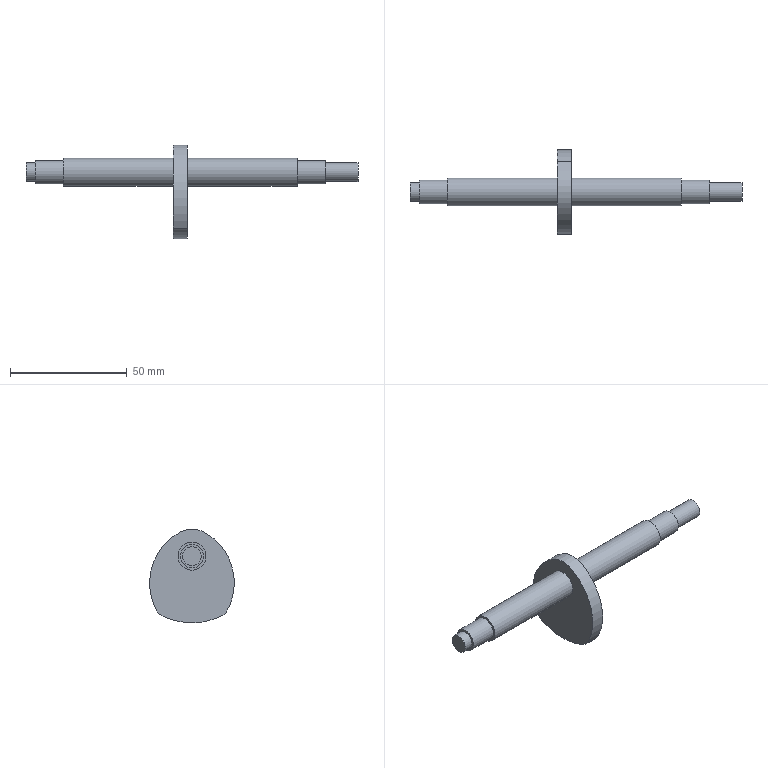Part | NX | features DATUM_CSYS 2, EXTRUDE 1, SKETCH 1, SWP104 1 | 1 solid | 16 faces | box 142 x 36.204 x 40.001 mm | volume 20323 mm3 | plane 8 | cylinder 6 | spline 2 | commonest cylinder face diameters 8 x2 10 x2 12 x2
STEP:
#1=CARTESIAN_POINT('',(-71.,0.,4.));
#2=VERTEX_POINT('',#1);
#3=CARTESIAN_POINT('',(-71.,0.,0.));
#4=DIRECTION('',(-1.,0.,0.));
#5=DIRECTION('',(0.,0.,1.));
#6=AXIS2_PLACEMENT_3D('',#3,#4,#5);
#7=CIRCLE('',#6,4.);
#8=EDGE_CURVE('',#2,#2,#7,.T.);
#9=ORIENTED_EDGE('',*,*,#8,.T.);
#10=EDGE_LOOP('',(#9));
#11=FACE_BOUND('',#10,.T.);
#12=CARTESIAN_POINT('',(-71.,0.,4.));
#13=DIRECTION('',(1.,0.,0.));
#14=DIRECTION('',(0.,0.,-1.));
#15=AXIS2_PLACEMENT_3D('',#12,#13,#14);
#16=PLANE('',#15);
#17=ADVANCED_FACE('',(#11),#16,.F.);
#18=CARTESIAN_POINT('',(-8.,0.,6.));
#19=VERTEX_POINT('',#18);
#20=CARTESIAN_POINT('',(-8.,0.,0.));
#21=DIRECTION('',(-1.,0.,0.));
#22=DIRECTION('',(0.,0.,1.));
#23=AXIS2_PLACEMENT_3D('',#20,#21,#22);
#24=CIRCLE('',#23,6.);
#25=EDGE_CURVE('',#19,#19,#24,.T.);
#26=ORIENTED_EDGE('',*,*,#25,.T.);
#27=EDGE_LOOP('',(#26));
#28=FACE_BOUND('',#27,.T.);
#29=CARTESIAN_POINT('',(-55.,0.,6.));
#30=VERTEX_POINT('',#29);
#31=CARTESIAN_POINT('',(-55.,0.,0.));
#32=DIRECTION('',(-1.,0.,0.));
#33=DIRECTION('',(0.,0.,1.));
#34=AXIS2_PLACEMENT_3D('',#31,#32,#33);
#35=CIRCLE('',#34,6.);
#36=EDGE_CURVE('',#30,#30,#35,.T.);
#37=ORIENTED_EDGE('',*,*,#36,.F.);
#38=EDGE_LOOP('',(#37));
#39=FACE_BOUND('',#38,.T.);
#40=CARTESIAN_POINT('',(71.,0.,0.));
#41=DIRECTION('',(-1.,0.,0.));
#42=DIRECTION('',(0.,0.,1.));
#43=AXIS2_PLACEMENT_3D('',#40,#41,#42);
#44=CYLINDRICAL_SURFACE('',#43,6.);
#45=ADVANCED_FACE('',(#28,#39),#44,.T.);
#46=CARTESIAN_POINT('',(-55.,0.,5.));
#47=VERTEX_POINT('',#46);
#48=CARTESIAN_POINT('',(-55.,0.,0.));
#49=DIRECTION('',(-1.,0.,0.));
#50=DIRECTION('',(0.,0.,1.));
#51=AXIS2_PLACEMENT_3D('',#48,#49,#50);
#52=CIRCLE('',#51,5.);
#53=EDGE_CURVE('',#47,#47,#52,.T.);
#54=ORIENTED_EDGE('',*,*,#53,.F.);
#55=EDGE_LOOP('',(#54));
#56=FACE_BOUND('',#55,.T.);
#57=ORIENTED_EDGE('',*,*,#36,.T.);
#58=EDGE_LOOP('',(#57));
#59=FACE_BOUND('',#58,.T.);
#60=CARTESIAN_POINT('',(-55.,0.,6.));
#61=DIRECTION('',(1.,0.,0.));
#62=DIRECTION('',(0.,0.,-1.));
#63=AXIS2_PLACEMENT_3D('',#60,#61,#62);
#64=PLANE('',#63);
#65=ADVANCED_FACE('',(#56,#59),#64,.F.);
#66=CARTESIAN_POINT('',(-67.,0.,5.));
#67=VERTEX_POINT('',#66);
#68=CARTESIAN_POINT('',(-67.,0.,0.));
#69=DIRECTION('',(-1.,0.,0.));
#70=DIRECTION('',(0.,0.,1.));
#71=AXIS2_PLACEMENT_3D('',#68,#69,#70);
#72=CIRCLE('',#71,5.);
#73=EDGE_CURVE('',#67,#67,#72,.T.);
#74=ORIENTED_EDGE('',*,*,#73,.F.);
#75=EDGE_LOOP('',(#74));
#76=FACE_BOUND('',#75,.T.);
#77=ORIENTED_EDGE('',*,*,#53,.T.);
#78=EDGE_LOOP('',(#77));
#79=FACE_BOUND('',#78,.T.);
#80=CARTESIAN_POINT('',(71.,0.,0.));
#81=DIRECTION('',(-1.,0.,0.));
#82=DIRECTION('',(0.,0.,1.));
#83=AXIS2_PLACEMENT_3D('',#80,#81,#82);
#84=CYLINDRICAL_SURFACE('',#83,5.);
#85=ADVANCED_FACE('',(#76,#79),#84,.T.);
#86=CARTESIAN_POINT('',(-67.,0.,4.));
#87=VERTEX_POINT('',#86);
#88=CARTESIAN_POINT('',(-67.,0.,0.));
#89=DIRECTION('',(-1.,0.,0.));
#90=DIRECTION('',(0.,0.,1.));
#91=AXIS2_PLACEMENT_3D('',#88,#89,#90);
#92=CIRCLE('',#91,4.);
#93=EDGE_CURVE('',#87,#87,#92,.T.);
#94=ORIENTED_EDGE('',*,*,#93,.F.);
#95=EDGE_LOOP('',(#94));
#96=FACE_BOUND('',#95,.T.);
#97=ORIENTED_EDGE('',*,*,#73,.T.);
#98=EDGE_LOOP('',(#97));
#99=FACE_BOUND('',#98,.T.);
#100=CARTESIAN_POINT('',(-67.,0.,5.));
#101=DIRECTION('',(1.,0.,0.));
#102=DIRECTION('',(0.,0.,-1.));
#103=AXIS2_PLACEMENT_3D('',#100,#101,#102);
#104=PLANE('',#103);
#105=ADVANCED_FACE('',(#96,#99),#104,.F.);
#106=ORIENTED_EDGE('',*,*,#8,.F.);
#107=EDGE_LOOP('',(#106));
#108=FACE_BOUND('',#107,.T.);
#109=ORIENTED_EDGE('',*,*,#93,.T.);
#110=EDGE_LOOP('',(#109));
#111=FACE_BOUND('',#110,.T.);
#112=CARTESIAN_POINT('',(71.,0.,0.));
#113=DIRECTION('',(-1.,0.,0.));
#114=DIRECTION('',(0.,0.,1.));
#115=AXIS2_PLACEMENT_3D('',#112,#113,#114);
#116=CYLINDRICAL_SURFACE('',#115,4.);
#117=ADVANCED_FACE('',(#108,#111),#116,.T.);
#118=CARTESIAN_POINT('',(-2.,12.9,3.729));
#119=VERTEX_POINT('',#118);
#120=CARTESIAN_POINT('',(-2.,-14.626,-23.983));
#121=VERTEX_POINT('',#120);
#122=CARTESIAN_POINT('',(-2.,12.9,3.729));
#123=CARTESIAN_POINT('',(-2.,12.125,4.726));
#124=CARTESIAN_POINT('',(-2.,10.846,6.133));
#125=CARTESIAN_POINT('',(-2.,8.942,7.797));
#126=CARTESIAN_POINT('',(-2.,7.802,8.648));
#127=CARTESIAN_POINT('',(-2.,7.017,9.178));
#128=CARTESIAN_POINT('',(-2.,6.487,9.522));
#129=CARTESIAN_POINT('',(-2.,5.813,9.933));
#130=CARTESIAN_POINT('',(-2.,5.115,10.304));
#131=CARTESIAN_POINT('',(-2.,4.541,10.568));
#132=CARTESIAN_POINT('',(-2.,3.663,10.926));
#133=CARTESIAN_POINT('',(-2.,2.293,11.322));
#134=CARTESIAN_POINT('',(-2.,0.4048,11.545));
#135=CARTESIAN_POINT('',(-2.,-1.495,11.455));
#136=CARTESIAN_POINT('',(-2.,-3.354,11.056));
#137=CARTESIAN_POINT('',(-2.,-4.826,10.468));
#138=CARTESIAN_POINT('',(-2.,-5.935,9.862));
#139=CARTESIAN_POINT('',(-2.,-6.607,9.446));
#140=CARTESIAN_POINT('',(-2.,-7.928,8.58));
#141=CARTESIAN_POINT('',(-2.,-9.933,7.033));
#142=CARTESIAN_POINT('',(-2.,-12.471,4.42));
#143=CARTESIAN_POINT('',(-2.,-14.668,1.318));
#144=CARTESIAN_POINT('',(-2.,-16.369,-2.082));
#145=CARTESIAN_POINT('',(-2.,-17.527,-5.703));
#146=CARTESIAN_POINT('',(-2.,-18.121,-9.458));
#147=CARTESIAN_POINT('',(-2.,-18.131,-13.259));
#148=CARTESIAN_POINT('',(-2.,-17.563,-17.018));
#149=CARTESIAN_POINT('',(-2.,-16.615,-20.041));
#150=CARTESIAN_POINT('',(-2.,-15.715,-22.062));
#151=CARTESIAN_POINT('',(-2.,-15.208,-23.045));
#152=CARTESIAN_POINT('',(-2.,-14.941,-23.529));
#153=CARTESIAN_POINT('',(-2.,-14.767,-23.793));
#154=CARTESIAN_POINT('',(-2.,-14.674,-23.921));
#155=CARTESIAN_POINT('',(-2.,-14.626,-23.983));
#156=B_SPLINE_CURVE_WITH_KNOTS('',3,(#122,#123,#124,#125,#126,#127,#128,#129,#130,#131,#132,#133,#134,#135,#136,#137,#138,#139,#140,#141,#142,#143,#144,#145,#146,#147,#148,#149,#150,#151,#152,#153,#154,#155),.UNSPECIFIED.,.F.,.F.,(4,1,1,1,1,1,1,1,1,1,1,1,1,1,1,1,1,1,1,1,1,1,1,1,1,1,1,1,1,1,1,4),(0.,0.0625,0.09375,0.125,0.1328,0.1406,0.1562,0.1719,0.1797,0.1875,0.2188,0.25,0.2812,0.3125,0.3438,0.3594,0.375,0.3828,0.4375,0.5,0.5625,0.625,0.6875,0.75,0.8125,0.875,0.9375,0.9688,0.9844,0.9922,0.9961,1.),.UNSPECIFIED.);
#157=EDGE_CURVE('',#119,#121,#156,.T.);
#158=ORIENTED_EDGE('',*,*,#157,.F.);
#159=CARTESIAN_POINT('',(-8.,12.9,3.729));
#160=VERTEX_POINT('',#159);
#161=CARTESIAN_POINT('',(-8.,12.9,3.729));
#162=DIRECTION('',(1.,0.,0.));
#163=VECTOR('',#162,1000.);
#164=LINE('',#161,#163);
#165=EDGE_CURVE('',#119,#160,#164,.F.);
#166=ORIENTED_EDGE('',*,*,#165,.T.);
#167=CARTESIAN_POINT('',(-8.,-14.626,-23.983));
#168=VERTEX_POINT('',#167);
#169=CARTESIAN_POINT('',(-8.,12.9,3.729));
#170=CARTESIAN_POINT('',(-8.,12.125,4.726));
#171=CARTESIAN_POINT('',(-8.,10.846,6.133));
#172=CARTESIAN_POINT('',(-8.,8.942,7.797));
#173=CARTESIAN_POINT('',(-8.,7.802,8.648));
#174=CARTESIAN_POINT('',(-8.,7.017,9.178));
#175=CARTESIAN_POINT('',(-8.,6.487,9.522));
#176=CARTESIAN_POINT('',(-8.,5.813,9.933));
#177=CARTESIAN_POINT('',(-8.,5.115,10.304));
#178=CARTESIAN_POINT('',(-8.,4.541,10.568));
#179=CARTESIAN_POINT('',(-8.,3.663,10.926));
#180=CARTESIAN_POINT('',(-8.,2.293,11.322));
#181=CARTESIAN_POINT('',(-8.,0.4048,11.545));
#182=CARTESIAN_POINT('',(-8.,-1.495,11.455));
#183=CARTESIAN_POINT('',(-8.,-3.354,11.056));
#184=CARTESIAN_POINT('',(-8.,-4.826,10.468));
#185=CARTESIAN_POINT('',(-8.,-5.935,9.862));
#186=CARTESIAN_POINT('',(-8.,-6.607,9.446));
#187=CARTESIAN_POINT('',(-8.,-7.928,8.58));
#188=CARTESIAN_POINT('',(-8.,-9.933,7.033));
#189=CARTESIAN_POINT('',(-8.,-12.471,4.42));
#190=CARTESIAN_POINT('',(-8.,-14.668,1.318));
#191=CARTESIAN_POINT('',(-8.,-16.369,-2.082));
#192=CARTESIAN_POINT('',(-8.,-17.527,-5.703));
#193=CARTESIAN_POINT('',(-8.,-18.121,-9.458));
#194=CARTESIAN_POINT('',(-8.,-18.131,-13.259));
#195=CARTESIAN_POINT('',(-8.,-17.563,-17.018));
#196=CARTESIAN_POINT('',(-8.,-16.615,-20.041));
#197=CARTESIAN_POINT('',(-8.,-15.715,-22.062));
#198=CARTESIAN_POINT('',(-8.,-15.208,-23.045));
#199=CARTESIAN_POINT('',(-8.,-14.941,-23.529));
#200=CARTESIAN_POINT('',(-8.,-14.767,-23.793));
#201=CARTESIAN_POINT('',(-8.,-14.674,-23.921));
#202=CARTESIAN_POINT('',(-8.,-14.626,-23.983));
#203=B_SPLINE_CURVE_WITH_KNOTS('',3,(#169,#170,#171,#172,#173,#174,#175,#176,#177,#178,#179,#180,#181,#182,#183,#184,#185,#186,#187,#188,#189,#190,#191,#192,#193,#194,#195,#196,#197,#198,#199,#200,#201,#202),.UNSPECIFIED.,.F.,.F.,(4,1,1,1,1,1,1,1,1,1,1,1,1,1,1,1,1,1,1,1,1,1,1,1,1,1,1,1,1,1,1,4),(0.,0.0625,0.09375,0.125,0.1328,0.1406,0.1562,0.1719,0.1797,0.1875,0.2188,0.25,0.2812,0.3125,0.3438,0.3594,0.375,0.3828,0.4375,0.5,0.5625,0.625,0.6875,0.75,0.8125,0.875,0.9375,0.9688,0.9844,0.9922,0.9961,1.),.UNSPECIFIED.);
#204=EDGE_CURVE('',#160,#168,#203,.T.);
#205=ORIENTED_EDGE('',*,*,#204,.T.);
#206=CARTESIAN_POINT('',(-8.,-14.626,-23.983));
#207=DIRECTION('',(1.,0.,0.));
#208=VECTOR('',#207,1000.);
#209=LINE('',#206,#208);
#210=EDGE_CURVE('',#168,#121,#209,.T.);
#211=ORIENTED_EDGE('',*,*,#210,.T.);
#212=EDGE_LOOP('',(#158,#166,#205,#211));
#213=FACE_BOUND('',#212,.T.);
#214=CARTESIAN_POINT('',(-8.,12.9,3.729));
#215=CARTESIAN_POINT('',(-2.,12.9,3.729));
#216=CARTESIAN_POINT('',(-8.,11.349,5.724));
#217=CARTESIAN_POINT('',(-2.,11.349,5.724));
#218=CARTESIAN_POINT('',(-8.,8.556,8.329));
#219=CARTESIAN_POINT('',(-2.,8.556,8.329));
#220=CARTESIAN_POINT('',(-8.,4.183,10.945));
#221=CARTESIAN_POINT('',(-2.,4.183,10.945));
#222=CARTESIAN_POINT('',(-8.,0.4114,11.698));
#223=CARTESIAN_POINT('',(-2.,0.4114,11.698));
#224=CARTESIAN_POINT('',(-8.,-3.411,11.221));
#225=CARTESIAN_POINT('',(-2.,-3.411,11.221));
#226=CARTESIAN_POINT('',(-8.,-6.799,9.446));
#227=CARTESIAN_POINT('',(-2.,-6.799,9.446));
#228=CARTESIAN_POINT('',(-8.,-9.82,7.146));
#229=CARTESIAN_POINT('',(-2.,-9.82,7.146));
#230=CARTESIAN_POINT('',(-8.,-13.355,3.512));
#231=CARTESIAN_POINT('',(-2.,-13.355,3.512));
#232=CARTESIAN_POINT('',(-8.,-16.64,-1.972));
#233=CARTESIAN_POINT('',(-2.,-16.64,-1.972));
#234=CARTESIAN_POINT('',(-8.,-18.117,-8.19));
#235=CARTESIAN_POINT('',(-2.,-18.117,-8.19));
#236=CARTESIAN_POINT('',(-8.,-18.132,-13.26));
#237=CARTESIAN_POINT('',(-2.,-18.132,-13.26));
#238=CARTESIAN_POINT('',(-8.,-17.561,-17.016));
#239=CARTESIAN_POINT('',(-2.,-17.561,-17.016));
#240=CARTESIAN_POINT('',(-8.,-16.621,-20.045));
#241=CARTESIAN_POINT('',(-2.,-16.621,-20.045));
#242=CARTESIAN_POINT('',(-8.,-15.575,-22.343));
#243=CARTESIAN_POINT('',(-2.,-15.575,-22.343));
#244=CARTESIAN_POINT('',(-8.,-15.01,-23.481));
#245=CARTESIAN_POINT('',(-2.,-15.01,-23.481));
#246=CARTESIAN_POINT('',(-8.,-14.626,-23.983));
#247=CARTESIAN_POINT('',(-2.,-14.626,-23.983));
#248=B_SPLINE_SURFACE_WITH_KNOTS('',3,1,((#214,#215),(#216,#217),(#218,#219),(#220,#221),(#222,#223),(#224,#225),(#226,#227),(#228,#229),(#230,#231),(#232,#233),(#234,#235),(#236,#237),(#238,#239),(#240,#241),(#242,#243),(#244,#245),(#246,#247)),.SURF_OF_LINEAR_EXTRUSION.,.F.,.F.,.F.,(4,1,1,1,1,1,1,1,1,1,1,1,1,1,4),(2,2),(0.,0.125,0.1875,0.25,0.3125,0.375,0.4375,0.5,0.625,0.75,0.8125,0.875,0.9375,0.9688,1.),(0.,1.),.UNSPECIFIED.);
#249=ADVANCED_FACE('',(#213),#248,.T.);
#250=CARTESIAN_POINT('',(-2.,-14.626,-23.983));
#251=CARTESIAN_POINT('',(-2.,-14.434,-24.235));
#252=CARTESIAN_POINT('',(-2.,-14.001,-24.701));
#253=CARTESIAN_POINT('',(-2.,-13.36,-25.172));
#254=CARTESIAN_POINT('',(-2.,-12.861,-25.436));
#255=CARTESIAN_POINT('',(-2.,-12.576,-25.575));
#256=CARTESIAN_POINT('',(-2.,-12.371,-25.675));
#257=CARTESIAN_POINT('',(-2.,-12.166,-25.773));
#258=CARTESIAN_POINT('',(-2.,-11.879,-25.907));
#259=CARTESIAN_POINT('',(-2.,-10.499,-26.53));
#260=CARTESIAN_POINT('',(-2.,-6.77,-27.888));
#261=CARTESIAN_POINT('',(-2.,-0.45,-28.837));
#262=CARTESIAN_POINT('',(-2.,5.897,-28.085));
#263=CARTESIAN_POINT('',(-2.,9.817,-26.795));
#264=CARTESIAN_POINT('',(-2.,11.493,-26.084));
#265=CARTESIAN_POINT('',(-2.,12.069,-25.82));
#266=CARTESIAN_POINT('',(-2.,12.497,-25.614));
#267=CARTESIAN_POINT('',(-2.,12.854,-25.441));
#268=CARTESIAN_POINT('',(-2.,13.411,-25.141));
#269=CARTESIAN_POINT('',(-2.,14.046,-24.66));
#270=CARTESIAN_POINT('',(-2.,14.58,-24.071));
#271=CARTESIAN_POINT('',(-2.,14.934,-23.545));
#272=CARTESIAN_POINT('',(-2.,15.389,-22.71));
#273=CARTESIAN_POINT('',(-2.,16.296,-20.861));
#274=CARTESIAN_POINT('',(-2.,17.352,-17.864));
#275=CARTESIAN_POINT('',(-2.,18.053,-14.117));
#276=CARTESIAN_POINT('',(-2.,18.175,-10.307));
#277=CARTESIAN_POINT('',(-2.,17.708,-6.524));
#278=CARTESIAN_POINT('',(-2.,16.67,-2.856));
#279=CARTESIAN_POINT('',(-2.,15.078,0.6081));
#280=CARTESIAN_POINT('',(-2.,13.678,2.729));
#281=CARTESIAN_POINT('',(-2.,12.9,3.729));
#282=B_SPLINE_CURVE_WITH_KNOTS('',3,(#250,#251,#252,#253,#254,#255,#256,#257,#258,#259,#260,#261,#262,#263,#264,#265,#266,#267,#268,#269,#270,#271,#272,#273,#274,#275,#276,#277,#278,#279,#280,#281),.UNSPECIFIED.,.F.,.F.,(4,1,1,1,1,1,1,1,1,1,1,1,1,1,1,1,1,1,1,1,1,1,1,1,1,1,1,1,1,4),(0.,0.01562,0.03125,0.03906,0.04346,0.04688,0.05029,0.05469,0.0625,0.125,0.25,0.375,0.4375,0.4531,0.4648,0.4688,0.4766,0.4844,0.5,0.5156,0.5234,0.5312,0.5625,0.625,0.6875,0.75,0.8125,0.875,0.9375,1.),.UNSPECIFIED.);
#283=EDGE_CURVE('',#121,#119,#282,.T.);
#284=ORIENTED_EDGE('',*,*,#283,.F.);
#285=ORIENTED_EDGE('',*,*,#210,.F.);
#286=CARTESIAN_POINT('',(-8.,-14.626,-23.983));
#287=CARTESIAN_POINT('',(-8.,-14.434,-24.235));
#288=CARTESIAN_POINT('',(-8.,-14.001,-24.701));
#289=CARTESIAN_POINT('',(-8.,-13.36,-25.172));
#290=CARTESIAN_POINT('',(-8.,-12.861,-25.436));
#291=CARTESIAN_POINT('',(-8.,-12.576,-25.575));
#292=CARTESIAN_POINT('',(-8.,-12.371,-25.675));
#293=CARTESIAN_POINT('',(-8.,-12.166,-25.773));
#294=CARTESIAN_POINT('',(-8.,-11.879,-25.907));
#295=CARTESIAN_POINT('',(-8.,-10.499,-26.53));
#296=CARTESIAN_POINT('',(-8.,-6.77,-27.888));
#297=CARTESIAN_POINT('',(-8.,-0.45,-28.837));
#298=CARTESIAN_POINT('',(-8.,5.897,-28.085));
#299=CARTESIAN_POINT('',(-8.,9.817,-26.795));
#300=CARTESIAN_POINT('',(-8.,11.493,-26.084));
#301=CARTESIAN_POINT('',(-8.,12.069,-25.82));
#302=CARTESIAN_POINT('',(-8.,12.497,-25.614));
#303=CARTESIAN_POINT('',(-8.,12.854,-25.441));
#304=CARTESIAN_POINT('',(-8.,13.411,-25.141));
#305=CARTESIAN_POINT('',(-8.,14.046,-24.66));
#306=CARTESIAN_POINT('',(-8.,14.58,-24.071));
#307=CARTESIAN_POINT('',(-8.,14.934,-23.545));
#308=CARTESIAN_POINT('',(-8.,15.389,-22.71));
#309=CARTESIAN_POINT('',(-8.,16.296,-20.861));
#310=CARTESIAN_POINT('',(-8.,17.352,-17.864));
#311=CARTESIAN_POINT('',(-8.,18.053,-14.117));
#312=CARTESIAN_POINT('',(-8.,18.175,-10.307));
#313=CARTESIAN_POINT('',(-8.,17.708,-6.524));
#314=CARTESIAN_POINT('',(-8.,16.67,-2.856));
#315=CARTESIAN_POINT('',(-8.,15.078,0.6081));
#316=CARTESIAN_POINT('',(-8.,13.678,2.729));
#317=CARTESIAN_POINT('',(-8.,12.9,3.729));
#318=B_SPLINE_CURVE_WITH_KNOTS('',3,(#286,#287,#288,#289,#290,#291,#292,#293,#294,#295,#296,#297,#298,#299,#300,#301,#302,#303,#304,#305,#306,#307,#308,#309,#310,#311,#312,#313,#314,#315,#316,#317),.UNSPECIFIED.,.F.,.F.,(4,1,1,1,1,1,1,1,1,1,1,1,1,1,1,1,1,1,1,1,1,1,1,1,1,1,1,1,1,4),(0.,0.01562,0.03125,0.03906,0.04346,0.04688,0.05029,0.05469,0.0625,0.125,0.25,0.375,0.4375,0.4531,0.4648,0.4688,0.4766,0.4844,0.5,0.5156,0.5234,0.5312,0.5625,0.625,0.6875,0.75,0.8125,0.875,0.9375,1.),.UNSPECIFIED.);
#319=EDGE_CURVE('',#168,#160,#318,.T.);
#320=ORIENTED_EDGE('',*,*,#319,.T.);
#321=ORIENTED_EDGE('',*,*,#165,.F.);
#322=EDGE_LOOP('',(#284,#285,#320,#321));
#323=FACE_BOUND('',#322,.T.);
#324=CARTESIAN_POINT('',(-8.,-14.626,-23.983));
#325=CARTESIAN_POINT('',(-2.,-14.626,-23.983));
#326=CARTESIAN_POINT('',(-8.,-13.857,-24.99));
#327=CARTESIAN_POINT('',(-2.,-13.857,-24.99));
#328=CARTESIAN_POINT('',(-8.,-11.513,-26.142));
#329=CARTESIAN_POINT('',(-2.,-11.513,-26.142));
#330=CARTESIAN_POINT('',(-8.,-7.971,-27.456));
#331=CARTESIAN_POINT('',(-2.,-7.971,-27.456));
#332=CARTESIAN_POINT('',(-8.,-4.24,-28.267));
#333=CARTESIAN_POINT('',(-2.,-4.24,-28.267));
#334=CARTESIAN_POINT('',(-8.,-0.4467,-28.582));
#335=CARTESIAN_POINT('',(-2.,-0.4467,-28.582));
#336=CARTESIAN_POINT('',(-8.,3.358,-28.386));
#337=CARTESIAN_POINT('',(-2.,3.358,-28.386));
#338=CARTESIAN_POINT('',(-8.,7.102,-27.69));
#339=CARTESIAN_POINT('',(-2.,7.102,-27.69));
#340=CARTESIAN_POINT('',(-8.,10.12,-26.692));
#341=CARTESIAN_POINT('',(-2.,10.12,-26.692));
#342=CARTESIAN_POINT('',(-8.,12.432,-25.675));
#343=CARTESIAN_POINT('',(-2.,12.432,-25.675));
#344=CARTESIAN_POINT('',(-8.,14.13,-24.752));
#345=CARTESIAN_POINT('',(-2.,14.13,-24.752));
#346=CARTESIAN_POINT('',(-8.,15.205,-23.145));
#347=CARTESIAN_POINT('',(-2.,15.205,-23.145));
#348=CARTESIAN_POINT('',(-8.,16.281,-20.856));
#349=CARTESIAN_POINT('',(-2.,16.281,-20.856));
#350=CARTESIAN_POINT('',(-8.,17.357,-17.866));
#351=CARTESIAN_POINT('',(-2.,17.357,-17.866));
#352=CARTESIAN_POINT('',(-8.,18.052,-14.117));
#353=CARTESIAN_POINT('',(-2.,18.052,-14.117));
#354=CARTESIAN_POINT('',(-8.,18.216,-9.037));
#355=CARTESIAN_POINT('',(-2.,18.216,-9.037));
#356=CARTESIAN_POINT('',(-8.,16.946,-2.754));
#357=CARTESIAN_POINT('',(-2.,16.946,-2.754));
#358=CARTESIAN_POINT('',(-8.,14.456,1.729));
#359=CARTESIAN_POINT('',(-2.,14.456,1.729));
#360=CARTESIAN_POINT('',(-8.,12.9,3.729));
#361=CARTESIAN_POINT('',(-2.,12.9,3.729));
#362=B_SPLINE_SURFACE_WITH_KNOTS('',3,1,((#324,#325),(#326,#327),(#328,#329),(#330,#331),(#332,#333),(#334,#335),(#336,#337),(#338,#339),(#340,#341),(#342,#343),(#344,#345),(#346,#347),(#348,#349),(#350,#351),(#352,#353),(#354,#355),(#356,#357),(#358,#359),(#360,#361)),.SURF_OF_LINEAR_EXTRUSION.,.F.,.F.,.F.,(4,1,1,1,1,1,1,1,1,1,1,1,1,1,1,1,4),(2,2),(0.,0.0625,0.125,0.1875,0.25,0.3125,0.375,0.4375,0.4688,0.5,0.5312,0.5625,0.625,0.6875,0.75,0.875,1.),(0.,1.),.UNSPECIFIED.);
#363=ADVANCED_FACE('',(#323),#362,.T.);
#364=ORIENTED_EDGE('',*,*,#25,.F.);
#365=EDGE_LOOP('',(#364));
#366=FACE_BOUND('',#365,.T.);
#367=ORIENTED_EDGE('',*,*,#204,.F.);
#368=ORIENTED_EDGE('',*,*,#319,.F.);
#369=EDGE_LOOP('',(#367,#368));
#370=FACE_BOUND('',#369,.T.);
#371=CARTESIAN_POINT('',(-8.,-12.396,4.357));
#372=DIRECTION('',(-1.,0.,0.));
#373=DIRECTION('',(0.,0.,1.));
#374=AXIS2_PLACEMENT_3D('',#371,#372,#373);
#375=PLANE('',#374);
#376=ADVANCED_FACE('',(#366,#370),#375,.T.);
#377=CARTESIAN_POINT('',(-2.,0.,6.));
#378=VERTEX_POINT('',#377);
#379=CARTESIAN_POINT('',(-2.,0.,0.));
#380=DIRECTION('',(-1.,0.,0.));
#381=DIRECTION('',(0.,0.,1.));
#382=AXIS2_PLACEMENT_3D('',#379,#380,#381);
#383=CIRCLE('',#382,6.);
#384=EDGE_CURVE('',#378,#378,#383,.T.);
#385=ORIENTED_EDGE('',*,*,#384,.T.);
#386=EDGE_LOOP('',(#385));
#387=FACE_BOUND('',#386,.T.);
#388=ORIENTED_EDGE('',*,*,#157,.T.);
#389=ORIENTED_EDGE('',*,*,#283,.T.);
#390=EDGE_LOOP('',(#388,#389));
#391=FACE_BOUND('',#390,.T.);
#392=CARTESIAN_POINT('',(-2.,-12.396,4.357));
#393=DIRECTION('',(-1.,0.,0.));
#394=DIRECTION('',(0.,0.,1.));
#395=AXIS2_PLACEMENT_3D('',#392,#393,#394);
#396=PLANE('',#395);
#397=ADVANCED_FACE('',(#387,#391),#396,.F.);
#398=CARTESIAN_POINT('',(71.,0.,4.));
#399=VERTEX_POINT('',#398);
#400=CARTESIAN_POINT('',(71.,0.,0.));
#401=DIRECTION('',(-1.,0.,0.));
#402=DIRECTION('',(0.,0.,1.));
#403=AXIS2_PLACEMENT_3D('',#400,#401,#402);
#404=CIRCLE('',#403,4.);
#405=EDGE_CURVE('',#399,#399,#404,.T.);
#406=ORIENTED_EDGE('',*,*,#405,.F.);
#407=EDGE_LOOP('',(#406));
#408=FACE_BOUND('',#407,.T.);
#409=CARTESIAN_POINT('',(71.,0.,0.));
#410=DIRECTION('',(-1.,0.,0.));
#411=DIRECTION('',(0.,0.,1.));
#412=AXIS2_PLACEMENT_3D('',#409,#410,#411);
#413=PLANE('',#412);
#414=ADVANCED_FACE('',(#408),#413,.F.);
#415=CARTESIAN_POINT('',(57.,0.,4.));
#416=VERTEX_POINT('',#415);
#417=CARTESIAN_POINT('',(57.,0.,0.));
#418=DIRECTION('',(-1.,0.,0.));
#419=DIRECTION('',(0.,0.,1.));
#420=AXIS2_PLACEMENT_3D('',#417,#418,#419);
#421=CIRCLE('',#420,4.);
#422=EDGE_CURVE('',#416,#416,#421,.T.);
#423=ORIENTED_EDGE('',*,*,#422,.F.);
#424=EDGE_LOOP('',(#423));
#425=FACE_BOUND('',#424,.T.);
#426=ORIENTED_EDGE('',*,*,#405,.T.);
#427=EDGE_LOOP('',(#426));
#428=FACE_BOUND('',#427,.T.);
#429=CARTESIAN_POINT('',(71.,0.,0.));
#430=DIRECTION('',(-1.,0.,0.));
#431=DIRECTION('',(0.,0.,1.));
#432=AXIS2_PLACEMENT_3D('',#429,#430,#431);
#433=CYLINDRICAL_SURFACE('',#432,4.);
#434=ADVANCED_FACE('',(#425,#428),#433,.T.);
#435=CARTESIAN_POINT('',(57.,0.,5.));
#436=VERTEX_POINT('',#435);
#437=CARTESIAN_POINT('',(57.,0.,0.));
#438=DIRECTION('',(-1.,0.,0.));
#439=DIRECTION('',(0.,0.,1.));
#440=AXIS2_PLACEMENT_3D('',#437,#438,#439);
#441=CIRCLE('',#440,5.);
#442=EDGE_CURVE('',#436,#436,#441,.T.);
#443=ORIENTED_EDGE('',*,*,#442,.F.);
#444=EDGE_LOOP('',(#443));
#445=FACE_BOUND('',#444,.T.);
#446=ORIENTED_EDGE('',*,*,#422,.T.);
#447=EDGE_LOOP('',(#446));
#448=FACE_BOUND('',#447,.T.);
#449=CARTESIAN_POINT('',(57.,0.,4.));
#450=DIRECTION('',(-1.,0.,0.));
#451=DIRECTION('',(0.,0.,1.));
#452=AXIS2_PLACEMENT_3D('',#449,#450,#451);
#453=PLANE('',#452);
#454=ADVANCED_FACE('',(#445,#448),#453,.F.);
#455=CARTESIAN_POINT('',(45.,0.,5.));
#456=VERTEX_POINT('',#455);
#457=CARTESIAN_POINT('',(45.,0.,0.));
#458=DIRECTION('',(-1.,0.,0.));
#459=DIRECTION('',(0.,0.,1.));
#460=AXIS2_PLACEMENT_3D('',#457,#458,#459);
#461=CIRCLE('',#460,5.);
#462=EDGE_CURVE('',#456,#456,#461,.T.);
#463=ORIENTED_EDGE('',*,*,#462,.F.);
#464=EDGE_LOOP('',(#463));
#465=FACE_BOUND('',#464,.T.);
#466=ORIENTED_EDGE('',*,*,#442,.T.);
#467=EDGE_LOOP('',(#466));
#468=FACE_BOUND('',#467,.T.);
#469=CARTESIAN_POINT('',(71.,0.,0.));
#470=DIRECTION('',(-1.,0.,0.));
#471=DIRECTION('',(0.,0.,1.));
#472=AXIS2_PLACEMENT_3D('',#469,#470,#471);
#473=CYLINDRICAL_SURFACE('',#472,5.);
#474=ADVANCED_FACE('',(#465,#468),#473,.T.);
#475=CARTESIAN_POINT('',(45.,0.,6.));
#476=VERTEX_POINT('',#475);
#477=CARTESIAN_POINT('',(45.,0.,0.));
#478=DIRECTION('',(-1.,0.,0.));
#479=DIRECTION('',(0.,0.,1.));
#480=AXIS2_PLACEMENT_3D('',#477,#478,#479);
#481=CIRCLE('',#480,6.);
#482=EDGE_CURVE('',#476,#476,#481,.T.);
#483=ORIENTED_EDGE('',*,*,#482,.F.);
#484=EDGE_LOOP('',(#483));
#485=FACE_BOUND('',#484,.T.);
#486=ORIENTED_EDGE('',*,*,#462,.T.);
#487=EDGE_LOOP('',(#486));
#488=FACE_BOUND('',#487,.T.);
#489=CARTESIAN_POINT('',(45.,0.,5.));
#490=DIRECTION('',(-1.,0.,0.));
#491=DIRECTION('',(0.,0.,1.));
#492=AXIS2_PLACEMENT_3D('',#489,#490,#491);
#493=PLANE('',#492);
#494=ADVANCED_FACE('',(#485,#488),#493,.F.);
#495=ORIENTED_EDGE('',*,*,#482,.T.);
#496=EDGE_LOOP('',(#495));
#497=FACE_BOUND('',#496,.T.);
#498=ORIENTED_EDGE('',*,*,#384,.F.);
#499=EDGE_LOOP('',(#498));
#500=FACE_BOUND('',#499,.T.);
#501=CARTESIAN_POINT('',(71.,0.,0.));
#502=DIRECTION('',(-1.,0.,0.));
#503=DIRECTION('',(0.,0.,1.));
#504=AXIS2_PLACEMENT_3D('',#501,#502,#503);
#505=CYLINDRICAL_SURFACE('',#504,6.);
#506=ADVANCED_FACE('',(#497,#500),#505,.T.);
#507=CLOSED_SHELL('',(#17,#45,#65,#85,#105,#117,#249,#363,#376,#397,#414,#434,#454,#474,#494,#506));
#508=MANIFOLD_SOLID_BREP('',#507);
#509=(LENGTH_UNIT()NAMED_UNIT(*)SI_UNIT(.MILLI.,.METRE.));
#510=UNCERTAINTY_MEASURE_WITH_UNIT(LENGTH_MEASURE(0.0508),#509,'','');
#511=(NAMED_UNIT(*)PLANE_ANGLE_UNIT()SI_UNIT($,.RADIAN.));
#512=(NAMED_UNIT(*)SI_UNIT($,.STERADIAN.)SOLID_ANGLE_UNIT());
#513=(GEOMETRIC_REPRESENTATION_CONTEXT(3)GLOBAL_UNCERTAINTY_ASSIGNED_CONTEXT((#510))GLOBAL_UNIT_ASSIGNED_CONTEXT((#509,#511,#512))REPRESENTATION_CONTEXT('',''));
#514=ADVANCED_BREP_SHAPE_REPRESENTATION('',(#508),#513);